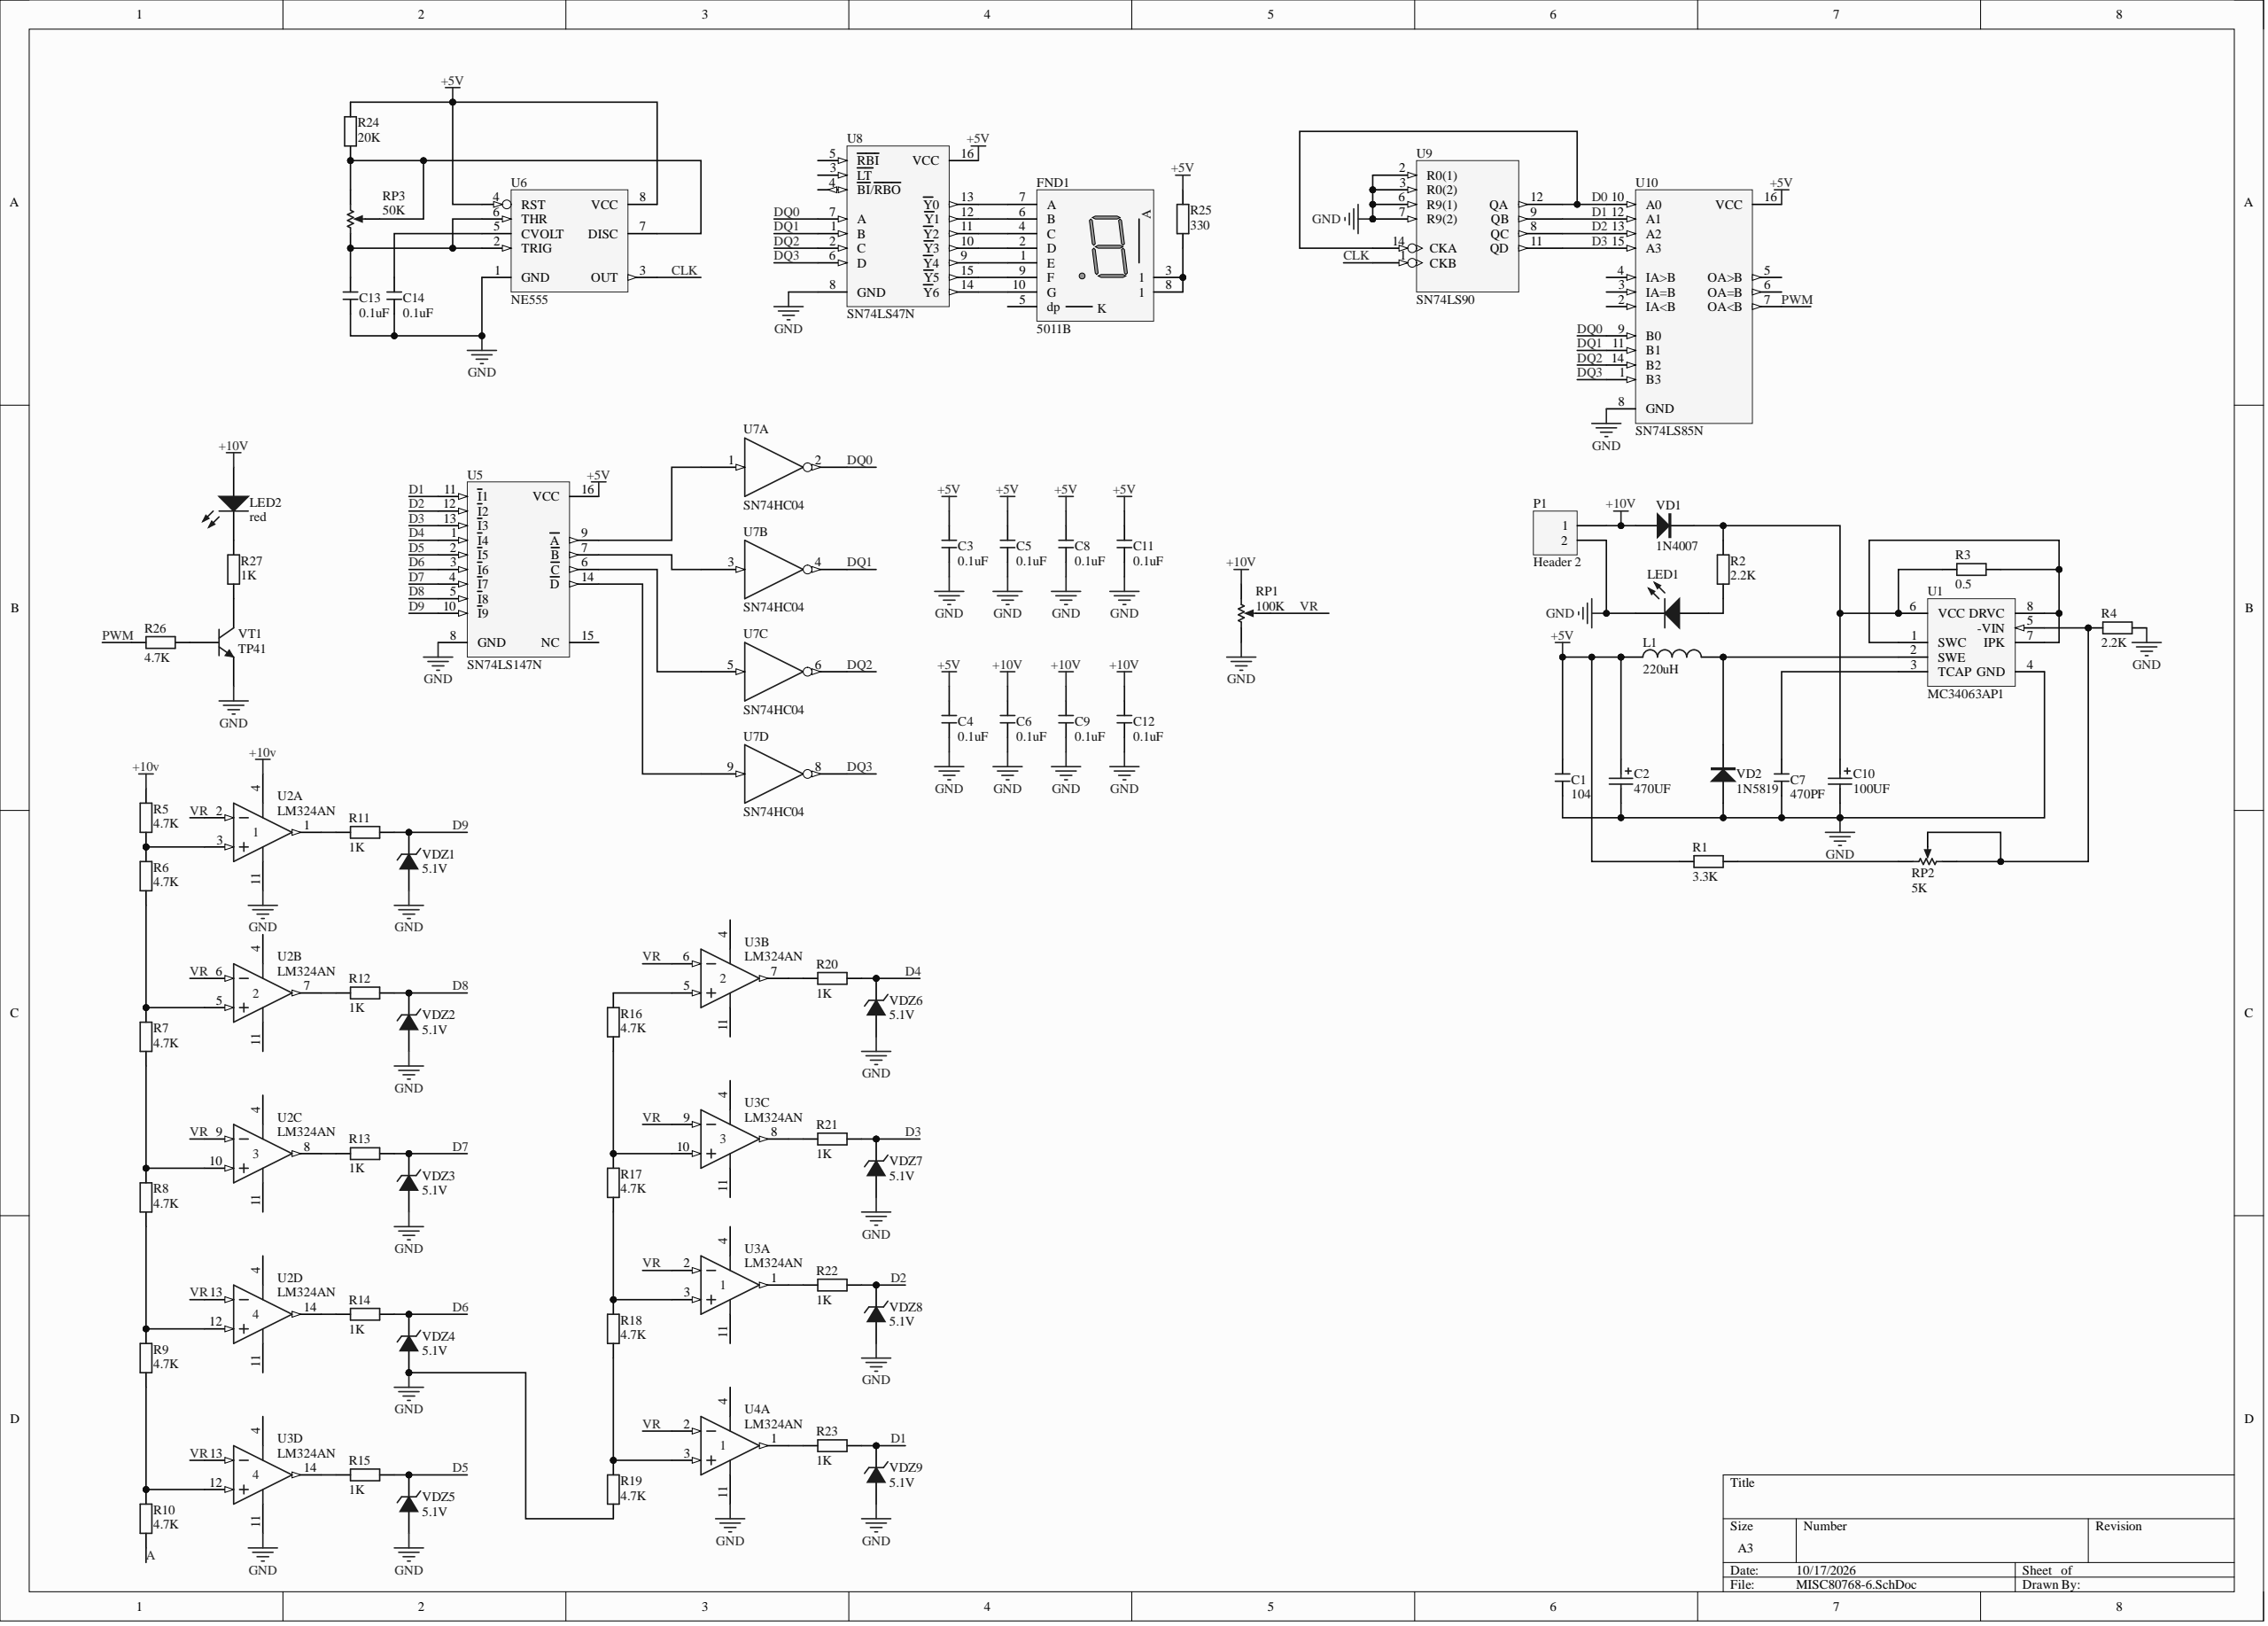Circuit board | Altium Designer | 71 parts | 64 nets
Bill of materials:
Comment,Description,Designator,Footprint,LibRef,Quantity
"104","ceramic capacitor","C1","CC 2.2*5","CC","1"
"470UF","Polarized Capacitor (Axial)","C2","CAP 1.5*4*8","Cap Pol2","1"
"0.1uF","ceramic capacitor","C3, C4, C5, C6, C8, C9, C11, C12, C13, C14","CC 2.2*5","CC","10"
"470PF","ceramic capacitor","C7","CC 2.2*5","CC","1"
"100UF","Polarized Capacitor (Axial)","C10","CAP 1.5*4*8","Cap Pol2","1"
"5011B","0.5 inch 1-digit common-anode seven-segment display","FND1","SMG 0.5-1P","5011B","1"
"220uH","color-band inductor","L1","AL0307","L-AL","1"
"red","3mm through-hole LED","LED1, LED2","LED 3MM-B","LED-3MM","2"
"Header 2","Header, 2-Pin","P1","HDR1X2","Header 2","1"
"3.3K","color-band resistor","R1","RS 1/4W","R-S","1"
"2.2K","color-band resistor","R2, R4","RS 1/4W","R-S","2"
"0.5","color-band resistor","R3","RS 1/4W","R-S","1"
"4.7K","color-band resistor","R5, R6, R7, R8, R9, R10, R16, R17, R18, R19, R26","RS 1/4W","R-S","11"
"1K","color-band resistor","R11, R12, R13, R14, R15, R20, R21, R22, R23, R27","RS 1/4W","R-S","10"
"20K","color-band resistor","R24","RS 1/4W","R-S","1"
"330","color-band resistor","R25","RS 1/4W","R-S","1"
"100K","Potentiometer","RP1","VR5","RPot","1"
"5K","Potentiometer","RP2","VR5","RPot","1"
"50K","Potentiometer","RP3","VR5","RPot","1"
"MC34063AP1","DC-to-DC Converter Control Circuit","U1","626-05","MC34063AP1","1"
"LM324AN","Quad Low-Power Operational Amplifier","U2, U3, U4","646-06","LM324AN","3"
"SN74LS147N","10-Line-to-4-Line Priority Encoder","U5","648-08","SN74LS147N","1"
"NE555","General-Purpose Single Bipolar Timer","U6","DIP8","NE555D","1"
"SN74HC04","Hex Inverters","U7","SO14","SN74HC04","1"
"SN74LS47N","BCD to 7-Segment Decoder/Driver","U8","648-08","SN74LS47N","1"
"SN74LS90","DECADE DIV-BY-12 BIN CNT","U9","DIP14","SN74LS90","1"
"SN74LS85N","4-Bit Magnitude Comparator","U10","648-08","SN74LS85N","1"
"1N4007","rectifier diode","VD1","DO-41","1N4007","1"
"1N5819","rectifier diode","VD2","DO-41","1N4007","1"
"5.1V","3V/0.5W zener diode","VDZ1, VDZ2, VDZ3, VDZ4, VDZ5, VDZ6, VDZ7, VDZ8, VDZ9","DO-35","1N4619","9"
"TP41","NPN General Purpose Amplifier","VT1","TO-92A","2N3904","1"
Netlist (Protel format):
[
C1
CC 2.2*5
104



]
[
C2
CAP 1.5*4*8
470UF



]
[
C3
CC 2.2*5
0.1uF



]
[
C4
CC 2.2*5
0.1uF



]
[
C5
CC 2.2*5
0.1uF



]
[
C6
CC 2.2*5
0.1uF



]
[
C7
CC 2.2*5
470PF



]
[
C8
CC 2.2*5
0.1uF



]
[
C9
CC 2.2*5
0.1uF



]
[
C10
CAP 1.5*4*8
100UF



]
[
C11
CC 2.2*5
0.1uF



]
[
C12
CC 2.2*5
0.1uF



]
[
C13
CC 2.2*5
0.1uF



]
[
C14
CC 2.2*5
0.1uF



]
[
FND1
SMG 0.5-1P
5011B



]
[
L1
AL0307
220uH



]
[
LED1
LED 3MM-B
red



]
[
LED2
LED 3MM-B
red



]
[
P1
HDR1X2
Header 2



]
[
R1
RS 1/4W
3.3K



]
[
R2
RS 1/4W
2.2K



]
[
R3
RS 1/4W
0.5



]
[
R4
RS 1/4W
2.2K



]
[
R5
RS 1/4W
4.7K



]
[
R6
RS 1/4W
4.7K



]
[
R7
RS 1/4W
4.7K



]
[
R8
RS 1/4W
4.7K



]
[
R9
RS 1/4W
4.7K



]
[
R10
RS 1/4W
4.7K



]
[
R11
RS 1/4W
1K



]
[
R12
RS 1/4W
1K



]
[
R13
RS 1/4W
1K



]
[
R14
RS 1/4W
1K



]
[
R15
RS 1/4W
1K



]
[
R16
RS 1/4W
4.7K



]
[
R17
RS 1/4W
4.7K



]
[
R18
RS 1/4W
4.7K



]
[
R19
RS 1/4W
4.7K



]
[
R20
RS 1/4W
1K



]
[
R21
RS 1/4W
1K



]
[
R22
RS 1/4W
1K



]
[
R23
RS 1/4W
1K



]
[
R24
RS 1/4W
20K



]
[
R25
RS 1/4W
330



]
[
R26
RS 1/4W
4.7K



]
[
R27
RS 1/4W
1K



]
[
RP1
VR5
100K



]
[
RP2
VR5
5K



]
[
RP3
VR5
50K



]
[
U1
626-05
MC34063AP1



]
[
U2
646-06
LM324AN



]
[
U3
646-06
LM324AN



]
[
U4
646-06
LM324AN



]
[
U5
648-08
SN74LS147N



]
[
U6
DIP8
NE555



]
[
U7
SO14
SN74HC04



]
[
U8
648-08
SN74LS47N



]
[
U9
DIP14
SN74LS90



]
[
U10
648-08
SN74LS85N



]
[
VD1
DO-41
1N4007



]
[
VD2
DO-41
1N5819



]
[
VDZ1
DO-35
5.1V



]
[
VDZ2
DO-35
5.1V



]
[
VDZ3
DO-35
5.1V



]
[
VDZ4
DO-35
5.1V



]
[
VDZ5
DO-35
5.1V



]
[
VDZ6
DO-35
5.1V



]
[
VDZ7
DO-35
5.1V



]
[
VDZ8
DO-35
5.1V



]
[
VDZ9
DO-35
5.1V



]
[
VT1
TO-92A
TP41



]
(
VR
RP1-3
U2-2
U2-6
U2-9
U2-13
U3-2
U3-6
U3-9
U3-13
U4-2
)
(
VCC
U7-14
U9-5
)
(
PWM
R26-2
U10-7
)
(
NetU5_14
U5-14
U7-9
)
(
NetU5_9
U5-9
U7-1
)
(
NetU5_7
U5-7
U7-3
)
(
NetU5_6
U5-6
U7-5
)
(
NetR27_1
R27-1
VT1-3
)
(
NetR26_1
R26-1
VT1-2
)
(
NetR24_1
R24-1
RP3-2
RP3-3
U6-7
)
(
NetR23_1
R23-1
U4-1
)
(
NetR22_1
R22-1
U3-1
)
(
NetR21_1
R21-1
U3-8
)
(
NetR20_1
R20-1
U3-7
)
(
NetR18_2
R18-2
R19-1
U4-3
)
(
NetR17_2
R17-2
R18-1
U3-3
)
(
NetR16_2
R16-2
R17-1
U3-10
)
(
NetR16_1
R16-1
U3-5
)
(
NetR15_1
R15-1
U3-14
)
(
NetR14_1
R14-1
U2-14
)
(
NetR13_1
R13-1
U2-8
)
(
NetR12_1
R12-1
U2-7
)
(
NetR11_1
R11-1
U2-1
)
(
NetR9_2
R9-2
R10-1
U3-12
)
(
NetR8_2
R8-2
R9-1
U2-12
)
(
NetR7_2
R7-2
R8-1
U2-10
)
(
NetR6_2
R6-2
R7-1
U2-5
)
(
NetR5_2
R5-2
R6-1
U2-3
)
(
NetR4_2
R4-2
RP2-1
RP2-3
U1-5
)
(
NetR3_1
R3-1
U1-1
U1-7
U1-8
)
(
NetR1_1
R1-1
RP2-2
)
(
NetLED2_2
LED2-2
R27-2
)
(
NetLED1_1
LED1-1
R2-1
)
(
NetL1_2
L1-2
U1-2
VD2-2
)
(
NetFND1_10
FND1-10
U8-14
)
(
NetFND1_9
FND1-9
U8-15
)
(
NetFND1_7
FND1-7
U8-13
)
(
NetFND1_6
FND1-6
U8-12
)
(
NetFND1_4
FND1-4
U8-11
)
(
NetFND1_3
FND1-3
FND1-8
R25-1
)
(
NetFND1_2
FND1-2
U8-10
)
(
NetFND1_1
FND1-1
U8-9
)
(
NetC14_1
C14-1
U6-5
)
(
NetC13_1
C13-1
RP3-1
U6-2
U6-6
)
(
NetC10_1
C10-1
R2-2
R3-2
U1-6
VD1-2
)
(
NetC7_1
C7-1
U1-3
)
(
GND
C1-2
C2-2
C3-2
C4-2
C5-2
C6-2
C7-2
C8-2
C9-2
C10-2
C11-2
C12-2
C13-2
C14-2
LED1-2
P1-2
R4-1
R19-2
RP1-1
U1-4
U2-11
U3-11
U4-11
U5-8
U6-1
U7-7
U8-8
U9-2
U9-3
U9-6
U9-7
U9-10
U10-8
VD2-1
VDZ1-1
VDZ2-1
VDZ3-1
VDZ4-1
VDZ5-1
VDZ6-1
VDZ7-1
VDZ8-1
VDZ9-1
VT1-1
)
(
DQ3
U7-8
U8-6
U10-1
)
(
DQ2
U7-6
U8-2
U10-14
)
(
DQ1
U7-4
U8-1
U10-11
)
(
DQ0
U7-2
U8-7
U10-9
)
(
D9
R11-2
U5-10
VDZ1-2
)
(
D8
R12-2
U5-5
VDZ2-2
)
(
D7
R13-2
U5-4
VDZ3-2
)
(
D6
R14-2
U5-3
VDZ4-2
)
(
D5
R15-2
U5-2
VDZ5-2
)
(
D4
R20-2
U5-1
VDZ6-2
)
(
D3
R21-2
U5-13
U9-11
U10-15
VDZ7-2
)
(
D2
R22-2
U5-12
U9-8
U10-13
VDZ8-2
)
(
D1
R23-2
U5-11
U9-9
U10-12
VDZ9-2
)
(
D0
U9-12
U9-14
U10-10
)
(
CLK
U6-3
U9-1
)
(
+10v
C6-1
C9-1
C12-1
LED2-1
P1-1
R5-1
RP1-2
U2-4
VD1-1
)
(
+5V
C1-1
C2-1
C3-1
C4-1
C5-1
C8-1
C11-1
L1-1
R1-2
R24-2
R25-2
U5-16
U6-4
U6-8
U8-16
U10-16
)